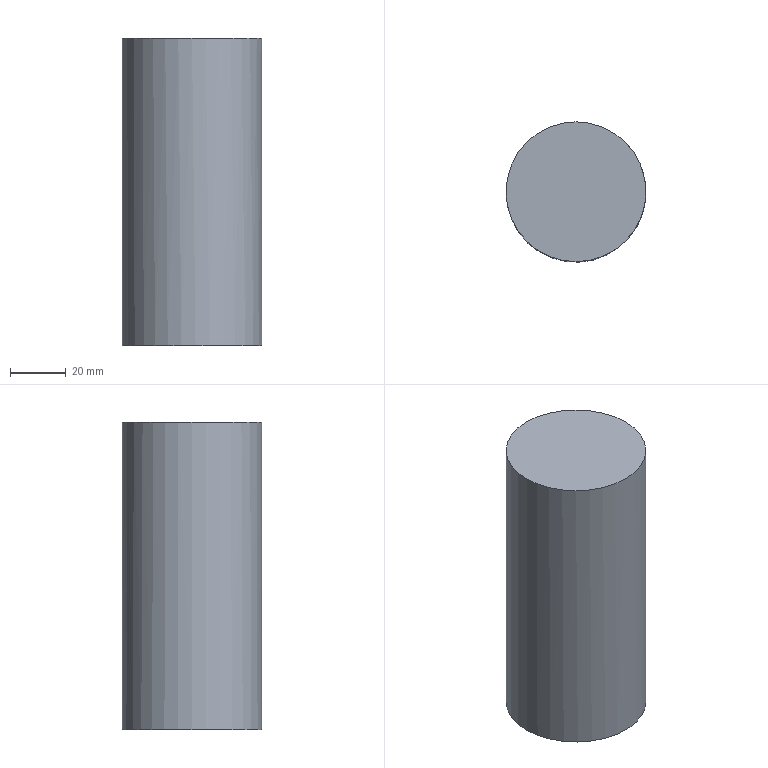Part | NX | features solid 2 | 1 solid | 3 faces | box 50 x 50 x 110 mm | volume 215984 mm3 | plane 2 | cylinder 1 | commonest cylinder face diameters 50 x1
STEP:
#1=CARTESIAN_POINT('',(1505.,470.,95.));
#2=VERTEX_POINT('',#1);
#3=CARTESIAN_POINT('',(1480.,470.,95.));
#4=DIRECTION('',(0.,0.,-1.));
#5=DIRECTION('',(1.,0.,0.));
#6=AXIS2_PLACEMENT_3D('',#3,#4,#5);
#7=CIRCLE('',#6,25.);
#8=EDGE_CURVE('',#2,#2,#7,.T.);
#9=ORIENTED_EDGE('',*,*,#8,.F.);
#10=EDGE_LOOP('',(#9));
#11=FACE_BOUND('',#10,.T.);
#12=CARTESIAN_POINT('',(1480.,470.,95.));
#13=DIRECTION('',(0.,0.,1.));
#14=DIRECTION('',(-1.,0.,0.));
#15=AXIS2_PLACEMENT_3D('',#12,#13,#14);
#16=PLANE('',#15);
#17=ADVANCED_FACE('',(#11),#16,.T.);
#18=CARTESIAN_POINT('',(1455.,470.,-15.));
#19=VERTEX_POINT('',#18);
#20=CARTESIAN_POINT('',(1480.,470.,-15.));
#21=DIRECTION('',(0.,0.,1.));
#22=DIRECTION('',(-1.,0.,0.));
#23=AXIS2_PLACEMENT_3D('',#20,#21,#22);
#24=CIRCLE('',#23,25.);
#25=EDGE_CURVE('',#19,#19,#24,.T.);
#26=ORIENTED_EDGE('',*,*,#25,.F.);
#27=EDGE_LOOP('',(#26));
#28=FACE_BOUND('',#27,.T.);
#29=CARTESIAN_POINT('',(1480.,470.,-15.));
#30=DIRECTION('',(0.,0.,-1.));
#31=DIRECTION('',(1.,0.,0.));
#32=AXIS2_PLACEMENT_3D('',#29,#30,#31);
#33=PLANE('',#32);
#34=ADVANCED_FACE('',(#28),#33,.T.);
#35=ORIENTED_EDGE('',*,*,#8,.T.);
#36=EDGE_LOOP('',(#35));
#37=FACE_BOUND('',#36,.T.);
#38=ORIENTED_EDGE('',*,*,#25,.T.);
#39=EDGE_LOOP('',(#38));
#40=FACE_BOUND('',#39,.T.);
#41=CARTESIAN_POINT('',(1480.,470.,-15.));
#42=DIRECTION('',(0.,0.,1.));
#43=DIRECTION('',(-1.,0.,0.));
#44=AXIS2_PLACEMENT_3D('',#41,#42,#43);
#45=CYLINDRICAL_SURFACE('',#44,25.);
#46=ADVANCED_FACE('',(#37,#40),#45,.T.);
#47=CLOSED_SHELL('',(#17,#34,#46));
#48=MANIFOLD_SOLID_BREP('',#47);
#49=(LENGTH_UNIT()NAMED_UNIT(*)SI_UNIT(.MILLI.,.METRE.));
#50=UNCERTAINTY_MEASURE_WITH_UNIT(LENGTH_MEASURE(0.00001),#49,'','');
#51=(NAMED_UNIT(*)PLANE_ANGLE_UNIT()SI_UNIT($,.RADIAN.));
#52=(NAMED_UNIT(*)SI_UNIT($,.STERADIAN.)SOLID_ANGLE_UNIT());
#53=(GEOMETRIC_REPRESENTATION_CONTEXT(3)GLOBAL_UNCERTAINTY_ASSIGNED_CONTEXT((#50))GLOBAL_UNIT_ASSIGNED_CONTEXT((#49,#51,#52))REPRESENTATION_CONTEXT('',''));
#54=ADVANCED_BREP_SHAPE_REPRESENTATION('',(#48),#53);